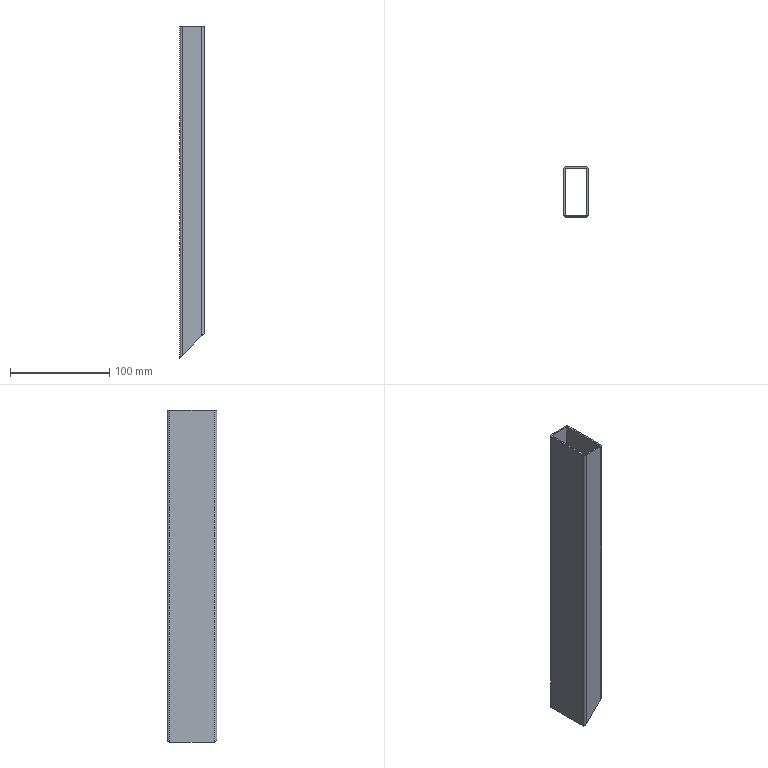Part | STEP file | 6150516 | 1 solid | 19 faces | box 25 x 50 x 334 mm | volume 67613 mm3 | plane 10 | cylinder 9 | commonest cylinder face diameters 2 x4 5 x4 18 x1
STEP:
#1=CARTESIAN_POINT('',(12.5,-22.5,25.));
#2=VERTEX_POINT('',#1);
#3=CARTESIAN_POINT('',(10.,-25.,22.5));
#4=VERTEX_POINT('',#3);
#5=CARTESIAN_POINT('',(12.5,-22.5,25.));
#6=CARTESIAN_POINT('',(12.5,-23.964,25.));
#7=CARTESIAN_POINT('',(11.464,-25.,23.964));
#8=CARTESIAN_POINT('',(10.,-25.,22.5));
#9=(BOUNDED_CURVE()B_SPLINE_CURVE(3,(#5,#6,#7,#8),.UNSPECIFIED.,.F.,.F.)B_SPLINE_CURVE_WITH_KNOTS((4,4),(3.142,4.712),.UNSPECIFIED.)CURVE()GEOMETRIC_REPRESENTATION_ITEM()RATIONAL_B_SPLINE_CURVE((1.,0.8047,0.8047,1.))REPRESENTATION_ITEM(''));
#10=EDGE_CURVE('',#2,#4,#9,.T.);
#11=ORIENTED_EDGE('',*,*,#10,.F.);
#12=CARTESIAN_POINT('',(12.5,-22.5,334.));
#13=VERTEX_POINT('',#12);
#14=CARTESIAN_POINT('',(12.5,-22.5,334.));
#15=DIRECTION('',(0.,0.,-1.));
#16=VECTOR('',#15,1000.);
#17=LINE('',#14,#16);
#18=EDGE_CURVE('',#13,#2,#17,.T.);
#19=ORIENTED_EDGE('',*,*,#18,.F.);
#20=CARTESIAN_POINT('',(10.,-25.,334.));
#21=VERTEX_POINT('',#20);
#22=CARTESIAN_POINT('',(10.,-22.5,334.));
#23=DIRECTION('',(0.,0.,1.));
#24=DIRECTION('',(1.,0.,0.));
#25=AXIS2_PLACEMENT_3D('',#22,#23,#24);
#26=CIRCLE('',#25,2.5);
#27=EDGE_CURVE('',#21,#13,#26,.T.);
#28=ORIENTED_EDGE('',*,*,#27,.F.);
#29=CARTESIAN_POINT('',(10.,-25.,334.));
#30=DIRECTION('',(0.,0.,-1.));
#31=VECTOR('',#30,1000.);
#32=LINE('',#29,#31);
#33=EDGE_CURVE('',#21,#4,#32,.T.);
#34=ORIENTED_EDGE('',*,*,#33,.T.);
#35=EDGE_LOOP('',(#11,#19,#28,#34));
#36=FACE_OUTER_BOUND('',#35,.T.);
#37=CARTESIAN_POINT('',(10.,-22.5,334.));
#38=DIRECTION('',(0.,0.,-1.));
#39=DIRECTION('',(-1.,0.,0.));
#40=AXIS2_PLACEMENT_3D('',#37,#38,#39);
#41=CYLINDRICAL_SURFACE('',#40,2.5);
#42=ADVANCED_FACE('',(#36),#41,.T.);
#43=CARTESIAN_POINT('',(12.5,11.,270.));
#44=VERTEX_POINT('',#43);
#45=CARTESIAN_POINT('',(12.5,2.,270.));
#46=DIRECTION('',(1.,0.,0.));
#47=DIRECTION('',(0.,1.,0.));
#48=AXIS2_PLACEMENT_3D('',#45,#46,#47);
#49=CIRCLE('',#48,9.);
#50=EDGE_CURVE('',#44,#44,#49,.T.);
#51=ORIENTED_EDGE('',*,*,#50,.F.);
#52=EDGE_LOOP('',(#51));
#53=FACE_BOUND('',#52,.T.);
#54=CARTESIAN_POINT('',(12.5,22.5,25.));
#55=VERTEX_POINT('',#54);
#56=CARTESIAN_POINT('',(12.5,22.5,25.));
#57=DIRECTION('',(0.,-1.,0.));
#58=VECTOR('',#57,1000.);
#59=LINE('',#56,#58);
#60=EDGE_CURVE('',#55,#2,#59,.T.);
#61=ORIENTED_EDGE('',*,*,#60,.F.);
#62=CARTESIAN_POINT('',(12.5,22.5,334.));
#63=VERTEX_POINT('',#62);
#64=CARTESIAN_POINT('',(12.5,22.5,334.));
#65=DIRECTION('',(0.,0.,-1.));
#66=VECTOR('',#65,1000.);
#67=LINE('',#64,#66);
#68=EDGE_CURVE('',#63,#55,#67,.T.);
#69=ORIENTED_EDGE('',*,*,#68,.F.);
#70=CARTESIAN_POINT('',(12.5,22.5,334.));
#71=DIRECTION('',(0.,1.,0.));
#72=VECTOR('',#71,1000.);
#73=LINE('',#70,#72);
#74=EDGE_CURVE('',#13,#63,#73,.T.);
#75=ORIENTED_EDGE('',*,*,#74,.F.);
#76=ORIENTED_EDGE('',*,*,#18,.T.);
#77=EDGE_LOOP('',(#61,#69,#75,#76));
#78=FACE_OUTER_BOUND('',#77,.T.);
#79=CARTESIAN_POINT('',(12.5,22.5,334.));
#80=DIRECTION('',(-1.,0.,0.));
#81=DIRECTION('',(0.,-1.,0.));
#82=AXIS2_PLACEMENT_3D('',#79,#80,#81);
#83=PLANE('',#82);
#84=ADVANCED_FACE('',(#53,#78),#83,.F.);
#85=CARTESIAN_POINT('',(10.,25.,22.5));
#86=VERTEX_POINT('',#85);
#87=CARTESIAN_POINT('',(10.,25.,22.5));
#88=CARTESIAN_POINT('',(11.464,25.,23.964));
#89=CARTESIAN_POINT('',(12.5,23.964,25.));
#90=CARTESIAN_POINT('',(12.5,22.5,25.));
#91=(BOUNDED_CURVE()B_SPLINE_CURVE(3,(#87,#88,#89,#90),.UNSPECIFIED.,.F.,.F.)B_SPLINE_CURVE_WITH_KNOTS((4,4),(1.571,3.142),.UNSPECIFIED.)CURVE()GEOMETRIC_REPRESENTATION_ITEM()RATIONAL_B_SPLINE_CURVE((1.,0.8047,0.8047,1.))REPRESENTATION_ITEM(''));
#92=EDGE_CURVE('',#86,#55,#91,.T.);
#93=ORIENTED_EDGE('',*,*,#92,.F.);
#94=CARTESIAN_POINT('',(10.,25.,334.));
#95=VERTEX_POINT('',#94);
#96=CARTESIAN_POINT('',(10.,25.,334.));
#97=DIRECTION('',(0.,0.,-1.));
#98=VECTOR('',#97,1000.);
#99=LINE('',#96,#98);
#100=EDGE_CURVE('',#95,#86,#99,.T.);
#101=ORIENTED_EDGE('',*,*,#100,.F.);
#102=CARTESIAN_POINT('',(10.,22.5,334.));
#103=DIRECTION('',(0.,0.,1.));
#104=DIRECTION('',(-1.,0.,0.));
#105=AXIS2_PLACEMENT_3D('',#102,#103,#104);
#106=CIRCLE('',#105,2.5);
#107=EDGE_CURVE('',#63,#95,#106,.T.);
#108=ORIENTED_EDGE('',*,*,#107,.F.);
#109=ORIENTED_EDGE('',*,*,#68,.T.);
#110=EDGE_LOOP('',(#93,#101,#108,#109));
#111=FACE_OUTER_BOUND('',#110,.T.);
#112=CARTESIAN_POINT('',(10.,22.5,334.));
#113=DIRECTION('',(0.,0.,-1.));
#114=DIRECTION('',(-1.,0.,0.));
#115=AXIS2_PLACEMENT_3D('',#112,#113,#114);
#116=CYLINDRICAL_SURFACE('',#115,2.5);
#117=ADVANCED_FACE('',(#111),#116,.T.);
#118=CARTESIAN_POINT('',(-10.,25.,2.5));
#119=VERTEX_POINT('',#118);
#120=CARTESIAN_POINT('',(155.75,25.,168.25));
#121=DIRECTION('',(0.7071,0.,0.7071));
#122=VECTOR('',#121,1000.);
#123=LINE('',#120,#122);
#124=EDGE_CURVE('',#119,#86,#123,.T.);
#125=ORIENTED_EDGE('',*,*,#124,.F.);
#126=CARTESIAN_POINT('',(-10.,25.,334.));
#127=VERTEX_POINT('',#126);
#128=CARTESIAN_POINT('',(-10.,25.,334.));
#129=DIRECTION('',(0.,0.,-1.));
#130=VECTOR('',#129,1000.);
#131=LINE('',#128,#130);
#132=EDGE_CURVE('',#127,#119,#131,.T.);
#133=ORIENTED_EDGE('',*,*,#132,.F.);
#134=CARTESIAN_POINT('',(-10.,25.,334.));
#135=DIRECTION('',(-1.,0.,0.));
#136=VECTOR('',#135,1000.);
#137=LINE('',#134,#136);
#138=EDGE_CURVE('',#95,#127,#137,.T.);
#139=ORIENTED_EDGE('',*,*,#138,.F.);
#140=ORIENTED_EDGE('',*,*,#100,.T.);
#141=EDGE_LOOP('',(#125,#133,#139,#140));
#142=FACE_OUTER_BOUND('',#141,.T.);
#143=CARTESIAN_POINT('',(-10.,25.,334.));
#144=DIRECTION('',(0.,-1.,0.));
#145=DIRECTION('',(0.,0.,-1.));
#146=AXIS2_PLACEMENT_3D('',#143,#144,#145);
#147=PLANE('',#146);
#148=ADVANCED_FACE('',(#142),#147,.F.);
#149=CARTESIAN_POINT('',(-12.5,22.5,0.));
#150=VERTEX_POINT('',#149);
#151=CARTESIAN_POINT('',(-12.5,22.5,0.));
#152=CARTESIAN_POINT('',(-12.5,23.964,0.));
#153=CARTESIAN_POINT('',(-11.464,25.,1.036));
#154=CARTESIAN_POINT('',(-10.,25.,2.5));
#155=(BOUNDED_CURVE()B_SPLINE_CURVE(3,(#151,#152,#153,#154),.UNSPECIFIED.,.F.,.T.)B_SPLINE_CURVE_WITH_KNOTS((4,4),(0.,1.571),.UNSPECIFIED.)CURVE()GEOMETRIC_REPRESENTATION_ITEM()RATIONAL_B_SPLINE_CURVE((1.,0.8047,0.8047,1.))REPRESENTATION_ITEM(''));
#156=EDGE_CURVE('',#150,#119,#155,.T.);
#157=ORIENTED_EDGE('',*,*,#156,.F.);
#158=CARTESIAN_POINT('',(-12.5,22.5,334.));
#159=VERTEX_POINT('',#158);
#160=CARTESIAN_POINT('',(-12.5,22.5,334.));
#161=DIRECTION('',(0.,0.,-1.));
#162=VECTOR('',#161,1000.);
#163=LINE('',#160,#162);
#164=EDGE_CURVE('',#159,#150,#163,.T.);
#165=ORIENTED_EDGE('',*,*,#164,.F.);
#166=CARTESIAN_POINT('',(-10.,22.5,334.));
#167=DIRECTION('',(0.,0.,1.));
#168=DIRECTION('',(1.,0.,0.));
#169=AXIS2_PLACEMENT_3D('',#166,#167,#168);
#170=CIRCLE('',#169,2.5);
#171=EDGE_CURVE('',#127,#159,#170,.T.);
#172=ORIENTED_EDGE('',*,*,#171,.F.);
#173=ORIENTED_EDGE('',*,*,#132,.T.);
#174=EDGE_LOOP('',(#157,#165,#172,#173));
#175=FACE_OUTER_BOUND('',#174,.T.);
#176=CARTESIAN_POINT('',(-10.,22.5,334.));
#177=DIRECTION('',(0.,0.,-1.));
#178=DIRECTION('',(-1.,0.,0.));
#179=AXIS2_PLACEMENT_3D('',#176,#177,#178);
#180=CYLINDRICAL_SURFACE('',#179,2.5);
#181=ADVANCED_FACE('',(#175),#180,.T.);
#182=CARTESIAN_POINT('',(-10.,-25.,2.5));
#183=VERTEX_POINT('',#182);
#184=CARTESIAN_POINT('',(-12.5,-22.5,0.));
#185=VERTEX_POINT('',#184);
#186=CARTESIAN_POINT('',(-10.,-25.,2.5));
#187=CARTESIAN_POINT('',(-11.464,-25.,1.036));
#188=CARTESIAN_POINT('',(-12.5,-23.964,0.));
#189=CARTESIAN_POINT('',(-12.5,-22.5,0.));
#190=(BOUNDED_CURVE()B_SPLINE_CURVE(3,(#186,#187,#188,#189),.UNSPECIFIED.,.F.,.T.)B_SPLINE_CURVE_WITH_KNOTS((4,4),(4.712,6.283),.UNSPECIFIED.)CURVE()GEOMETRIC_REPRESENTATION_ITEM()RATIONAL_B_SPLINE_CURVE((1.,0.8047,0.8047,1.))REPRESENTATION_ITEM(''));
#191=EDGE_CURVE('',#183,#185,#190,.T.);
#192=ORIENTED_EDGE('',*,*,#191,.F.);
#193=CARTESIAN_POINT('',(-10.,-25.,334.));
#194=VERTEX_POINT('',#193);
#195=CARTESIAN_POINT('',(-10.,-25.,334.));
#196=DIRECTION('',(0.,0.,-1.));
#197=VECTOR('',#196,1000.);
#198=LINE('',#195,#197);
#199=EDGE_CURVE('',#194,#183,#198,.T.);
#200=ORIENTED_EDGE('',*,*,#199,.F.);
#201=CARTESIAN_POINT('',(-12.5,-22.5,334.));
#202=VERTEX_POINT('',#201);
#203=CARTESIAN_POINT('',(-10.,-22.5,334.));
#204=DIRECTION('',(0.,0.,1.));
#205=DIRECTION('',(1.,0.,0.));
#206=AXIS2_PLACEMENT_3D('',#203,#204,#205);
#207=CIRCLE('',#206,2.5);
#208=EDGE_CURVE('',#202,#194,#207,.T.);
#209=ORIENTED_EDGE('',*,*,#208,.F.);
#210=CARTESIAN_POINT('',(-12.5,-22.5,334.));
#211=DIRECTION('',(0.,0.,-1.));
#212=VECTOR('',#211,1000.);
#213=LINE('',#210,#212);
#214=EDGE_CURVE('',#202,#185,#213,.T.);
#215=ORIENTED_EDGE('',*,*,#214,.T.);
#216=EDGE_LOOP('',(#192,#200,#209,#215));
#217=FACE_OUTER_BOUND('',#216,.T.);
#218=CARTESIAN_POINT('',(-10.,-22.5,334.));
#219=DIRECTION('',(0.,0.,-1.));
#220=DIRECTION('',(-1.,0.,0.));
#221=AXIS2_PLACEMENT_3D('',#218,#219,#220);
#222=CYLINDRICAL_SURFACE('',#221,2.5);
#223=ADVANCED_FACE('',(#217),#222,.T.);
#224=CARTESIAN_POINT('',(155.75,-25.,168.25));
#225=DIRECTION('',(-0.7071,0.,-0.7071));
#226=VECTOR('',#225,1000.);
#227=LINE('',#224,#226);
#228=EDGE_CURVE('',#4,#183,#227,.T.);
#229=ORIENTED_EDGE('',*,*,#228,.F.);
#230=ORIENTED_EDGE('',*,*,#33,.F.);
#231=CARTESIAN_POINT('',(-10.,-25.,334.));
#232=DIRECTION('',(1.,0.,0.));
#233=VECTOR('',#232,1000.);
#234=LINE('',#231,#233);
#235=EDGE_CURVE('',#194,#21,#234,.T.);
#236=ORIENTED_EDGE('',*,*,#235,.F.);
#237=ORIENTED_EDGE('',*,*,#199,.T.);
#238=EDGE_LOOP('',(#229,#230,#236,#237));
#239=FACE_OUTER_BOUND('',#238,.T.);
#240=CARTESIAN_POINT('',(-10.,-25.,334.));
#241=DIRECTION('',(0.,1.,0.));
#242=DIRECTION('',(-1.,0.,0.));
#243=AXIS2_PLACEMENT_3D('',#240,#241,#242);
#244=PLANE('',#243);
#245=ADVANCED_FACE('',(#239),#244,.F.);
#246=CARTESIAN_POINT('',(10.,23.5,334.));
#247=VERTEX_POINT('',#246);
#248=CARTESIAN_POINT('',(10.,23.5,22.5));
#249=VERTEX_POINT('',#248);
#250=CARTESIAN_POINT('',(10.,23.5,334.));
#251=DIRECTION('',(0.,0.,-1.));
#252=VECTOR('',#251,1000.);
#253=LINE('',#250,#252);
#254=EDGE_CURVE('',#247,#249,#253,.T.);
#255=ORIENTED_EDGE('',*,*,#254,.T.);
#256=CARTESIAN_POINT('',(11.,22.5,23.5));
#257=VERTEX_POINT('',#256);
#258=CARTESIAN_POINT('',(10.,23.5,22.5));
#259=CARTESIAN_POINT('',(10.586,23.5,23.086));
#260=CARTESIAN_POINT('',(11.,23.086,23.5));
#261=CARTESIAN_POINT('',(11.,22.5,23.5));
#262=(BOUNDED_CURVE()B_SPLINE_CURVE(3,(#258,#259,#260,#261),.UNSPECIFIED.,.F.,.F.)B_SPLINE_CURVE_WITH_KNOTS((4,4),(1.571,3.142),.UNSPECIFIED.)CURVE()GEOMETRIC_REPRESENTATION_ITEM()RATIONAL_B_SPLINE_CURVE((1.,0.8047,0.8047,1.))REPRESENTATION_ITEM(''));
#263=EDGE_CURVE('',#249,#257,#262,.T.);
#264=ORIENTED_EDGE('',*,*,#263,.T.);
#265=CARTESIAN_POINT('',(11.,22.5,334.));
#266=VERTEX_POINT('',#265);
#267=CARTESIAN_POINT('',(11.,22.5,334.));
#268=DIRECTION('',(0.,0.,-1.));
#269=VECTOR('',#268,1000.);
#270=LINE('',#267,#269);
#271=EDGE_CURVE('',#266,#257,#270,.T.);
#272=ORIENTED_EDGE('',*,*,#271,.F.);
#273=CARTESIAN_POINT('',(10.,22.5,334.));
#274=DIRECTION('',(0.,0.,1.));
#275=DIRECTION('',(-1.,0.,0.));
#276=AXIS2_PLACEMENT_3D('',#273,#274,#275);
#277=CIRCLE('',#276,1.);
#278=EDGE_CURVE('',#266,#247,#277,.T.);
#279=ORIENTED_EDGE('',*,*,#278,.T.);
#280=EDGE_LOOP('',(#255,#264,#272,#279));
#281=FACE_OUTER_BOUND('',#280,.T.);
#282=CARTESIAN_POINT('',(10.,22.5,334.));
#283=DIRECTION('',(0.,0.,-1.));
#284=DIRECTION('',(-1.,0.,0.));
#285=AXIS2_PLACEMENT_3D('',#282,#283,#284);
#286=CYLINDRICAL_SURFACE('',#285,1.);
#287=ADVANCED_FACE('',(#281),#286,.F.);
#288=CARTESIAN_POINT('',(-10.,23.5,334.));
#289=VERTEX_POINT('',#288);
#290=CARTESIAN_POINT('',(-10.,23.5,2.5));
#291=VERTEX_POINT('',#290);
#292=CARTESIAN_POINT('',(-10.,23.5,334.));
#293=DIRECTION('',(0.,0.,-1.));
#294=VECTOR('',#293,1000.);
#295=LINE('',#292,#294);
#296=EDGE_CURVE('',#289,#291,#295,.T.);
#297=ORIENTED_EDGE('',*,*,#296,.T.);
#298=CARTESIAN_POINT('',(155.75,23.5,168.25));
#299=DIRECTION('',(0.7071,0.,0.7071));
#300=VECTOR('',#299,1000.);
#301=LINE('',#298,#300);
#302=EDGE_CURVE('',#291,#249,#301,.T.);
#303=ORIENTED_EDGE('',*,*,#302,.T.);
#304=ORIENTED_EDGE('',*,*,#254,.F.);
#305=CARTESIAN_POINT('',(-10.,23.5,334.));
#306=DIRECTION('',(-1.,0.,0.));
#307=VECTOR('',#306,1000.);
#308=LINE('',#305,#307);
#309=EDGE_CURVE('',#247,#289,#308,.T.);
#310=ORIENTED_EDGE('',*,*,#309,.T.);
#311=EDGE_LOOP('',(#297,#303,#304,#310));
#312=FACE_OUTER_BOUND('',#311,.T.);
#313=CARTESIAN_POINT('',(-10.,23.5,334.));
#314=DIRECTION('',(0.,-1.,0.));
#315=DIRECTION('',(1.,0.,0.));
#316=AXIS2_PLACEMENT_3D('',#313,#314,#315);
#317=PLANE('',#316);
#318=ADVANCED_FACE('',(#312),#317,.T.);
#319=CARTESIAN_POINT('',(-11.,22.5,334.));
#320=VERTEX_POINT('',#319);
#321=CARTESIAN_POINT('',(-11.,22.5,1.5));
#322=VERTEX_POINT('',#321);
#323=CARTESIAN_POINT('',(-11.,22.5,334.));
#324=DIRECTION('',(0.,0.,-1.));
#325=VECTOR('',#324,1000.);
#326=LINE('',#323,#325);
#327=EDGE_CURVE('',#320,#322,#326,.T.);
#328=ORIENTED_EDGE('',*,*,#327,.T.);
#329=CARTESIAN_POINT('',(-11.,22.5,1.5));
#330=CARTESIAN_POINT('',(-11.,23.086,1.5));
#331=CARTESIAN_POINT('',(-10.586,23.5,1.914));
#332=CARTESIAN_POINT('',(-10.,23.5,2.5));
#333=(BOUNDED_CURVE()B_SPLINE_CURVE(3,(#329,#330,#331,#332),.UNSPECIFIED.,.F.,.F.)B_SPLINE_CURVE_WITH_KNOTS((4,4),(0.,1.571),.UNSPECIFIED.)CURVE()GEOMETRIC_REPRESENTATION_ITEM()RATIONAL_B_SPLINE_CURVE((1.,0.8047,0.8047,1.))REPRESENTATION_ITEM(''));
#334=EDGE_CURVE('',#322,#291,#333,.T.);
#335=ORIENTED_EDGE('',*,*,#334,.T.);
#336=ORIENTED_EDGE('',*,*,#296,.F.);
#337=CARTESIAN_POINT('',(-10.,22.5,334.));
#338=DIRECTION('',(0.,0.,1.));
#339=DIRECTION('',(1.,0.,0.));
#340=AXIS2_PLACEMENT_3D('',#337,#338,#339);
#341=CIRCLE('',#340,1.);
#342=EDGE_CURVE('',#289,#320,#341,.T.);
#343=ORIENTED_EDGE('',*,*,#342,.T.);
#344=EDGE_LOOP('',(#328,#335,#336,#343));
#345=FACE_OUTER_BOUND('',#344,.T.);
#346=CARTESIAN_POINT('',(-10.,22.5,334.));
#347=DIRECTION('',(0.,0.,-1.));
#348=DIRECTION('',(-1.,0.,0.));
#349=AXIS2_PLACEMENT_3D('',#346,#347,#348);
#350=CYLINDRICAL_SURFACE('',#349,1.);
#351=ADVANCED_FACE('',(#345),#350,.F.);
#352=CARTESIAN_POINT('',(-11.,-22.5,334.));
#353=VERTEX_POINT('',#352);
#354=CARTESIAN_POINT('',(-11.,-22.5,1.5));
#355=VERTEX_POINT('',#354);
#356=CARTESIAN_POINT('',(-11.,-22.5,334.));
#357=DIRECTION('',(0.,0.,-1.));
#358=VECTOR('',#357,1000.);
#359=LINE('',#356,#358);
#360=EDGE_CURVE('',#353,#355,#359,.T.);
#361=ORIENTED_EDGE('',*,*,#360,.T.);
#362=CARTESIAN_POINT('',(-11.,22.5,1.5));
#363=DIRECTION('',(0.,1.,0.));
#364=VECTOR('',#363,1000.);
#365=LINE('',#362,#364);
#366=EDGE_CURVE('',#355,#322,#365,.T.);
#367=ORIENTED_EDGE('',*,*,#366,.T.);
#368=ORIENTED_EDGE('',*,*,#327,.F.);
#369=CARTESIAN_POINT('',(-11.,22.5,334.));
#370=DIRECTION('',(0.,-1.,0.));
#371=VECTOR('',#370,1000.);
#372=LINE('',#369,#371);
#373=EDGE_CURVE('',#320,#353,#372,.T.);
#374=ORIENTED_EDGE('',*,*,#373,.T.);
#375=EDGE_LOOP('',(#361,#367,#368,#374));
#376=FACE_OUTER_BOUND('',#375,.T.);
#377=CARTESIAN_POINT('',(-11.,22.5,334.));
#378=DIRECTION('',(1.,0.,0.));
#379=DIRECTION('',(0.,1.,0.));
#380=AXIS2_PLACEMENT_3D('',#377,#378,#379);
#381=PLANE('',#380);
#382=ADVANCED_FACE('',(#376),#381,.T.);
#383=CARTESIAN_POINT('',(-10.,-23.5,334.));
#384=VERTEX_POINT('',#383);
#385=CARTESIAN_POINT('',(-10.,-23.5,2.5));
#386=VERTEX_POINT('',#385);
#387=CARTESIAN_POINT('',(-10.,-23.5,334.));
#388=DIRECTION('',(0.,0.,-1.));
#389=VECTOR('',#388,1000.);
#390=LINE('',#387,#389);
#391=EDGE_CURVE('',#384,#386,#390,.T.);
#392=ORIENTED_EDGE('',*,*,#391,.T.);
#393=CARTESIAN_POINT('',(-10.,-23.5,2.5));
#394=CARTESIAN_POINT('',(-10.586,-23.5,1.914));
#395=CARTESIAN_POINT('',(-11.,-23.086,1.5));
#396=CARTESIAN_POINT('',(-11.,-22.5,1.5));
#397=(BOUNDED_CURVE()B_SPLINE_CURVE(3,(#393,#394,#395,#396),.UNSPECIFIED.,.F.,.T.)B_SPLINE_CURVE_WITH_KNOTS((4,4),(4.712,6.283),.UNSPECIFIED.)CURVE()GEOMETRIC_REPRESENTATION_ITEM()RATIONAL_B_SPLINE_CURVE((1.,0.8047,0.8047,1.))REPRESENTATION_ITEM(''));
#398=EDGE_CURVE('',#386,#355,#397,.T.);
#399=ORIENTED_EDGE('',*,*,#398,.T.);
#400=ORIENTED_EDGE('',*,*,#360,.F.);
#401=CARTESIAN_POINT('',(-10.,-22.5,334.));
#402=DIRECTION('',(0.,0.,1.));
#403=DIRECTION('',(1.,0.,0.));
#404=AXIS2_PLACEMENT_3D('',#401,#402,#403);
#405=CIRCLE('',#404,1.);
#406=EDGE_CURVE('',#353,#384,#405,.T.);
#407=ORIENTED_EDGE('',*,*,#406,.T.);
#408=EDGE_LOOP('',(#392,#399,#400,#407));
#409=FACE_OUTER_BOUND('',#408,.T.);
#410=CARTESIAN_POINT('',(-10.,-22.5,334.));
#411=DIRECTION('',(0.,0.,-1.));
#412=DIRECTION('',(-1.,0.,0.));
#413=AXIS2_PLACEMENT_3D('',#410,#411,#412);
#414=CYLINDRICAL_SURFACE('',#413,1.);
#415=ADVANCED_FACE('',(#409),#414,.F.);
#416=CARTESIAN_POINT('',(10.,-23.5,334.));
#417=VERTEX_POINT('',#416);
#418=CARTESIAN_POINT('',(10.,-23.5,22.5));
#419=VERTEX_POINT('',#418);
#420=CARTESIAN_POINT('',(10.,-23.5,334.));
#421=DIRECTION('',(0.,0.,-1.));
#422=VECTOR('',#421,1000.);
#423=LINE('',#420,#422);
#424=EDGE_CURVE('',#417,#419,#423,.T.);
#425=ORIENTED_EDGE('',*,*,#424,.T.);
#426=CARTESIAN_POINT('',(155.75,-23.5,168.25));
#427=DIRECTION('',(-0.7071,0.,-0.7071));
#428=VECTOR('',#427,1000.);
#429=LINE('',#426,#428);
#430=EDGE_CURVE('',#419,#386,#429,.T.);
#431=ORIENTED_EDGE('',*,*,#430,.T.);
#432=ORIENTED_EDGE('',*,*,#391,.F.);
#433=CARTESIAN_POINT('',(-10.,-23.5,334.));
#434=DIRECTION('',(1.,0.,0.));
#435=VECTOR('',#434,1000.);
#436=LINE('',#433,#435);
#437=EDGE_CURVE('',#384,#417,#436,.T.);
#438=ORIENTED_EDGE('',*,*,#437,.T.);
#439=EDGE_LOOP('',(#425,#431,#432,#438));
#440=FACE_OUTER_BOUND('',#439,.T.);
#441=CARTESIAN_POINT('',(-10.,-23.5,334.));
#442=DIRECTION('',(0.,1.,0.));
#443=DIRECTION('',(0.,0.,1.));
#444=AXIS2_PLACEMENT_3D('',#441,#442,#443);
#445=PLANE('',#444);
#446=ADVANCED_FACE('',(#440),#445,.T.);
#447=CARTESIAN_POINT('',(11.,-22.5,334.));
#448=VERTEX_POINT('',#447);
#449=CARTESIAN_POINT('',(11.,-22.5,23.5));
#450=VERTEX_POINT('',#449);
#451=CARTESIAN_POINT('',(11.,-22.5,334.));
#452=DIRECTION('',(0.,0.,-1.));
#453=VECTOR('',#452,1000.);
#454=LINE('',#451,#453);
#455=EDGE_CURVE('',#448,#450,#454,.T.);
#456=ORIENTED_EDGE('',*,*,#455,.T.);
#457=CARTESIAN_POINT('',(11.,-22.5,23.5));
#458=CARTESIAN_POINT('',(11.,-23.086,23.5));
#459=CARTESIAN_POINT('',(10.586,-23.5,23.086));
#460=CARTESIAN_POINT('',(10.,-23.5,22.5));
#461=(BOUNDED_CURVE()B_SPLINE_CURVE(3,(#457,#458,#459,#460),.UNSPECIFIED.,.F.,.F.)B_SPLINE_CURVE_WITH_KNOTS((4,4),(3.142,4.712),.UNSPECIFIED.)CURVE()GEOMETRIC_REPRESENTATION_ITEM()RATIONAL_B_SPLINE_CURVE((1.,0.8047,0.8047,1.))REPRESENTATION_ITEM(''));
#462=EDGE_CURVE('',#450,#419,#461,.T.);
#463=ORIENTED_EDGE('',*,*,#462,.T.);
#464=ORIENTED_EDGE('',*,*,#424,.F.);
#465=CARTESIAN_POINT('',(10.,-22.5,334.));
#466=DIRECTION('',(0.,0.,1.));
#467=DIRECTION('',(1.,0.,0.));
#468=AXIS2_PLACEMENT_3D('',#465,#466,#467);
#469=CIRCLE('',#468,1.);
#470=EDGE_CURVE('',#417,#448,#469,.T.);
#471=ORIENTED_EDGE('',*,*,#470,.T.);
#472=EDGE_LOOP('',(#456,#463,#464,#471));
#473=FACE_OUTER_BOUND('',#472,.T.);
#474=CARTESIAN_POINT('',(10.,-22.5,334.));
#475=DIRECTION('',(0.,0.,-1.));
#476=DIRECTION('',(-1.,0.,0.));
#477=AXIS2_PLACEMENT_3D('',#474,#475,#476);
#478=CYLINDRICAL_SURFACE('',#477,1.);
#479=ADVANCED_FACE('',(#473),#478,.F.);
#480=CARTESIAN_POINT('',(11.,2.,279.));
#481=VERTEX_POINT('',#480);
#482=CARTESIAN_POINT('',(11.,2.,270.));
#483=DIRECTION('',(-1.,0.,0.));
#484=DIRECTION('',(0.,0.,1.));
#485=AXIS2_PLACEMENT_3D('',#482,#483,#484);
#486=CIRCLE('',#485,9.);
#487=EDGE_CURVE('',#481,#481,#486,.T.);
#488=ORIENTED_EDGE('',*,*,#487,.F.);
#489=EDGE_LOOP('',(#488));
#490=FACE_BOUND('',#489,.T.);
#491=ORIENTED_EDGE('',*,*,#271,.T.);
#492=CARTESIAN_POINT('',(11.,22.5,23.5));
#493=DIRECTION('',(0.,-1.,0.));
#494=VECTOR('',#493,1000.);
#495=LINE('',#492,#494);
#496=EDGE_CURVE('',#257,#450,#495,.T.);
#497=ORIENTED_EDGE('',*,*,#496,.T.);
#498=ORIENTED_EDGE('',*,*,#455,.F.);
#499=CARTESIAN_POINT('',(11.,22.5,334.));
#500=DIRECTION('',(0.,1.,0.));
#501=VECTOR('',#500,1000.);
#502=LINE('',#499,#501);
#503=EDGE_CURVE('',#448,#266,#502,.T.);
#504=ORIENTED_EDGE('',*,*,#503,.T.);
#505=EDGE_LOOP('',(#491,#497,#498,#504));
#506=FACE_OUTER_BOUND('',#505,.T.);
#507=CARTESIAN_POINT('',(11.,22.5,334.));
#508=DIRECTION('',(-1.,0.,0.));
#509=DIRECTION('',(0.,0.,1.));
#510=AXIS2_PLACEMENT_3D('',#507,#508,#509);
#511=PLANE('',#510);
#512=ADVANCED_FACE('',(#490,#506),#511,.T.);
#513=ORIENTED_EDGE('',*,*,#27,.T.);
#514=ORIENTED_EDGE('',*,*,#74,.T.);
#515=ORIENTED_EDGE('',*,*,#107,.T.);
#516=ORIENTED_EDGE('',*,*,#138,.T.);
#517=ORIENTED_EDGE('',*,*,#171,.T.);
#518=CARTESIAN_POINT('',(-12.5,22.5,334.));
#519=DIRECTION('',(0.,-1.,0.));
#520=VECTOR('',#519,1000.);
#521=LINE('',#518,#520);
#522=EDGE_CURVE('',#159,#202,#521,.T.);
#523=ORIENTED_EDGE('',*,*,#522,.T.);
#524=ORIENTED_EDGE('',*,*,#208,.T.);
#525=ORIENTED_EDGE('',*,*,#235,.T.);
#526=EDGE_LOOP('',(#513,#514,#515,#516,#517,#523,#524,#525));
#527=FACE_OUTER_BOUND('',#526,.T.);
#528=ORIENTED_EDGE('',*,*,#309,.F.);
#529=ORIENTED_EDGE('',*,*,#278,.F.);
#530=ORIENTED_EDGE('',*,*,#503,.F.);
#531=ORIENTED_EDGE('',*,*,#470,.F.);
#532=ORIENTED_EDGE('',*,*,#437,.F.);
#533=ORIENTED_EDGE('',*,*,#406,.F.);
#534=ORIENTED_EDGE('',*,*,#373,.F.);
#535=ORIENTED_EDGE('',*,*,#342,.F.);
#536=EDGE_LOOP('',(#528,#529,#530,#531,#532,#533,#534,#535));
#537=FACE_BOUND('',#536,.T.);
#538=CARTESIAN_POINT('',(10.,-22.5,334.));
#539=DIRECTION('',(0.,0.,1.));
#540=DIRECTION('',(1.,0.,0.));
#541=AXIS2_PLACEMENT_3D('',#538,#539,#540);
#542=PLANE('',#541);
#543=ADVANCED_FACE('',(#527,#537),#542,.T.);
#544=CARTESIAN_POINT('',(-12.5,22.5,0.));
#545=DIRECTION('',(0.,-1.,0.));
#546=VECTOR('',#545,1000.);
#547=LINE('',#544,#546);
#548=EDGE_CURVE('',#150,#185,#547,.T.);
#549=ORIENTED_EDGE('',*,*,#548,.T.);
#550=ORIENTED_EDGE('',*,*,#214,.F.);
#551=ORIENTED_EDGE('',*,*,#522,.F.);
#552=ORIENTED_EDGE('',*,*,#164,.T.);
#553=EDGE_LOOP('',(#549,#550,#551,#552));
#554=FACE_OUTER_BOUND('',#553,.T.);
#555=CARTESIAN_POINT('',(-12.5,22.5,334.));
#556=DIRECTION('',(1.,0.,0.));
#557=DIRECTION('',(0.,1.,0.));
#558=AXIS2_PLACEMENT_3D('',#555,#556,#557);
#559=PLANE('',#558);
#560=ADVANCED_FACE('',(#554),#559,.F.);
#561=ORIENTED_EDGE('',*,*,#263,.F.);
#562=ORIENTED_EDGE('',*,*,#302,.F.);
#563=ORIENTED_EDGE('',*,*,#334,.F.);
#564=ORIENTED_EDGE('',*,*,#366,.F.);
#565=ORIENTED_EDGE('',*,*,#398,.F.);
#566=ORIENTED_EDGE('',*,*,#430,.F.);
#567=ORIENTED_EDGE('',*,*,#462,.F.);
#568=ORIENTED_EDGE('',*,*,#496,.F.);
#569=EDGE_LOOP('',(#561,#562,#563,#564,#565,#566,#567,#568));
#570=FACE_BOUND('',#569,.T.);
#571=ORIENTED_EDGE('',*,*,#548,.F.);
#572=ORIENTED_EDGE('',*,*,#156,.T.);
#573=ORIENTED_EDGE('',*,*,#124,.T.);
#574=ORIENTED_EDGE('',*,*,#92,.T.);
#575=ORIENTED_EDGE('',*,*,#60,.T.);
#576=ORIENTED_EDGE('',*,*,#10,.T.);
#577=ORIENTED_EDGE('',*,*,#228,.T.);
#578=ORIENTED_EDGE('',*,*,#191,.T.);
#579=EDGE_LOOP('',(#571,#572,#573,#574,#575,#576,#577,#578));
#580=FACE_OUTER_BOUND('',#579,.T.);
#581=CARTESIAN_POINT('',(-12.5,507.682,0.));
#582=DIRECTION('',(0.7071,0.,-0.7071));
#583=DIRECTION('',(-0.7071,0.,-0.7071));
#584=AXIS2_PLACEMENT_3D('',#581,#582,#583);
#585=PLANE('',#584);
#586=ADVANCED_FACE('',(#570,#580),#585,.T.);
#587=ORIENTED_EDGE('',*,*,#487,.T.);
#588=EDGE_LOOP('',(#587));
#589=FACE_OUTER_BOUND('',#588,.T.);
#590=ORIENTED_EDGE('',*,*,#50,.T.);
#591=EDGE_LOOP('',(#590));
#592=FACE_OUTER_BOUND('',#591,.T.);
#593=CARTESIAN_POINT('',(2.5,2.,270.));
#594=DIRECTION('',(1.,0.,0.));
#595=DIRECTION('',(0.,1.,0.));
#596=AXIS2_PLACEMENT_3D('',#593,#594,#595);
#597=CYLINDRICAL_SURFACE('',#596,9.);
#598=ADVANCED_FACE('',(#589,#592),#597,.F.);
#599=CLOSED_SHELL('',(#42,#84,#117,#148,#181,#223,#245,#287,#318,#351,#382,#415,#446,#479,#512,#543,#560,#586,#598));
#600=MANIFOLD_SOLID_BREP('',#599);
#601=CARTESIAN_POINT('',(0.,0.,0.));
#602=DIRECTION('',(0.,0.,1.));
#603=DIRECTION('',(1.,0.,0.));
#604=AXIS2_PLACEMENT_3D('',#601,#602,#603);
#605=(LENGTH_UNIT()NAMED_UNIT(*)SI_UNIT(.MILLI.,.METRE.));
#606=UNCERTAINTY_MEASURE_WITH_UNIT(LENGTH_MEASURE(0.00001),#605,'','');
#607=(NAMED_UNIT(*)PLANE_ANGLE_UNIT()SI_UNIT($,.RADIAN.));
#608=(NAMED_UNIT(*)SI_UNIT($,.STERADIAN.)SOLID_ANGLE_UNIT());
#609=(GEOMETRIC_REPRESENTATION_CONTEXT(3)GLOBAL_UNCERTAINTY_ASSIGNED_CONTEXT((#606))GLOBAL_UNIT_ASSIGNED_CONTEXT((#605,#607,#608))REPRESENTATION_CONTEXT('',''));
#610=ADVANCED_BREP_SHAPE_REPRESENTATION('',(#600,#604),#609);